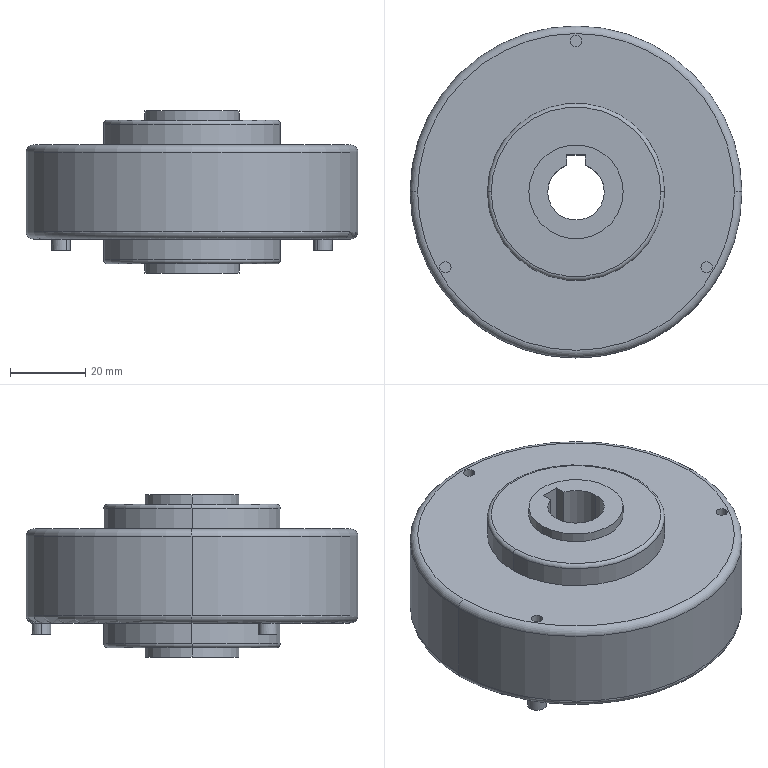Part | STEP file | YHD-LZ-PBN-0.3KG-yhd | 1 solid | 72 faces | box 88 x 88 x 43 mm | volume 168276 mm3 | plane 39 | cylinder 25 | torus 8 | commonest cylinder face diameters 3 x6 5 x6 25 x4 47 x4 15 x3 88 x2